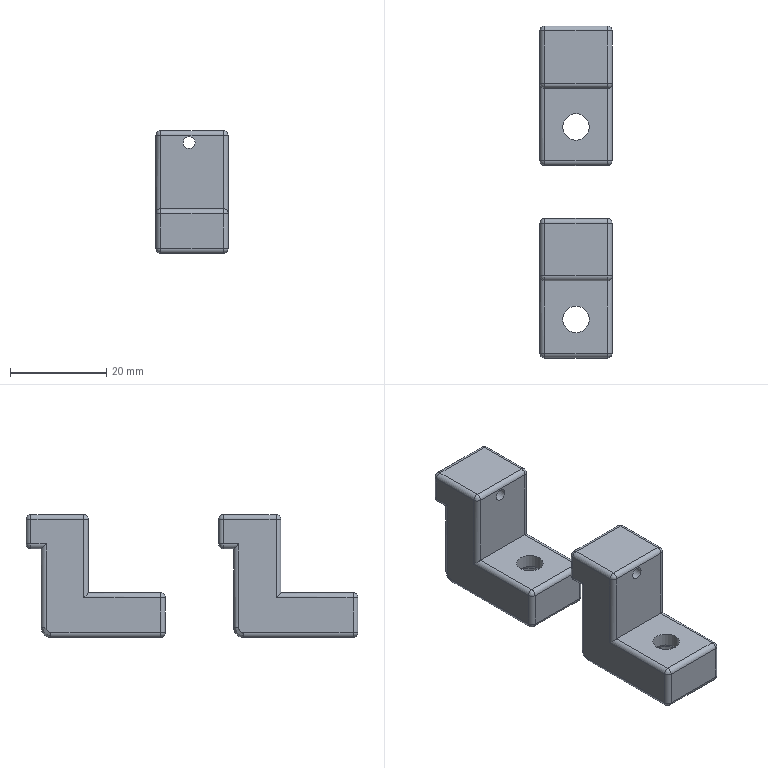CAM job | NX | 3-axis milling, drilling | part box 15 x 68.95 x 25.5 mm | stock box 20 x 73.95 x 30 mm
Tools:
number,name,description,diameter,corner_radius,flute_length,length,flutes
4,D4,平底铣刀-粗,4.0,0.0,25.0,75.0,2
6,D6,平底铣刀-粗,6.0,0.0,25.0,75.0,2
9,D10,平底铣刀-粗,10.0,0.0,35.0,75.0,2
7,D6-J,平底铣刀-精,6.0,0.0,25.0,75.0,2
18,D4R0.5,圆鼻刀-粗,4.0,0.5,50.0,75.0,2
1,D80R0.8飞刀,圆鼻刀-粗,80.0,0.8,50.0,75.0,2
1,D80R0.8飞刀-J,圆鼻刀-精,80.0,0.8,50.0,75.0,2
2,D6倒角刀,倒角刀,6.0,0.0,3.0,25.0,2
17,ZT5.5,钻头,5.5,0.0,35.0,50.0,2
Operations:
program,operation,operation_type,tool,method,geometry_group,spindle_rpm,surface_speed,feed_per_tooth,feed_cut,feed_plunge,cut_length_mm,path_length_mm,cut_time_min,machine_time_min
B,底壁铣飞面一刀开粗_COPY,VolumeBased25DMillingOperation,D80R0.8飞刀,分层开粗-切深K-步距G,W-B,2800.0,703.696,0.5357,3000.0,100.0,1594.679,3178.841,0.5316,0.69
B,底壁铣飞面一刀精光_COPY,VolumeBased25DMillingOperation,D80R0.8飞刀-J,侧刃精光-切深K-步距G,W-B,4000.0,1005.28,0.125,1000.0,100.0,176.99,212.99,0.177,0.1806
B,底壁铣分层开粗-中_COPY,VolumeBased25DMillingOperation,D10,分层开粗-切深K-步距G,W-B,8000.0,251.32,0.25,4000.0,100.0,7301.415,7478.472,1.825,1.843
B,等高螺旋爬面_COPY,ZLevelMilling,D4R0.5,等高爬面-切深K-步距G,W-B,7000.0,175.929,0.2857,4000.0,100.0,3123.524,3246.373,0.7809,0.7932
B,铣倒角_2,PlanarMilling,D6倒角刀,METHOD,W-B,8000.0,150.796,0.075,1200.0,100.0,35.589,225.483,0.0297,0.0486
B,底壁铣精光底面-中_COPY,VolumeBased25DMillingOperation,D6-J,精光步距切深关,W-B,7000.0,175.0,0.0536,1500.0,100.0,204.716,371.046,0.1365,0.1531
B,等高精光-中_COPY_1,ZLevelMilling,D6-J,侧刃精光-切深K-步距G,W-B,8000.0,150.792,0.0625,1000.0,100.0,123.039,377.209,0.123,0.1485
B,等高精光往复爬面_COPY_COPY_COPY_1,ZLevelMilling,D6-J,等高爬面-切深K-步距G,W-B,7000.0,87.965,0.3214,4500.0,100.0,1642.985,1808.549,0.3651,0.3817
A,顶面,FaceMilling,D80R0.8飞刀,侧刃精光-切深K-步距G,W-A,4000.0,1005.31,0.125,1000.0,100.0,162.95,198.95,0.1629,0.1665
A,外形粗_2,VolumeBased25DMillingOperation,D10,METHOD,W-A,8000.0,251.327,0.3125,5000.0,80.0,8042.542,8210.642,1.609,1.625
A,沉头孔打点-深0.8,Operation,D6倒角刀,NONE,W-A,8000.0,150.796,0.0312,500.0,90.0,3.6,88.213,0.0072,0.0157
A,沉头孔-钻孔0段,Operation,ZT5.5,NONE,W-A,1200.0,20.735,0.0625,150.0,90.0,27.805,136.622,0.1854,0.1962
A,底壁粗_1,VolumeBased25DMillingOperation,D4,METHOD,W-A,6000.0,56.549,0.0833,1000.0,100.0,6375.937,7477.18,6.376,6.486
A,铣孔开粗D6_1,CylinderMilling,D6,NONE,W-A,8000.0,150.796,0.075,1200.0,100.0,336.917,467.517,0.2808,0.2938
A,铣孔精光D6_1,CylinderMilling,D6,精光步距切深关,W-A,8000.0,150.796,0.0312,500.0,100.0,68.961,200.561,0.1379,0.1511
A,等高精光往复爬面_COPY,ZLevelMilling,D4R0.5,等高爬面-切深K-步距G,W-A,7000.0,87.965,0.3214,4500.0,100.0,3176.564,3261.452,0.7059,0.7144
A,等高精光往复爬面_COPY_COPY,ZLevelMilling,D4R0.5,等高爬面-切深K-步距G,W-A,7000.0,87.965,0.3214,4500.0,100.0,1874.539,1961.168,0.4166,0.4252
A,铣倒角_1,PlanarMilling,D6倒角刀,NONE,W-A,8000.0,150.796,0.05,800.0,100.0,80.502,196.93,0.1006,0.1123
A,等高精光-中_COPY,ZLevelMilling,D6-J,侧刃精光-切深K-步距G,W-A,8000.0,150.792,0.0625,1000.0,100.0,415.511,545.704,0.4155,0.4285
A,等高精光往复爬面_COPY_COPY_COPY,ZLevelMilling,D6-J,等高爬面-切深K-步距G,W-A,7000.0,87.965,0.3214,4500.0,100.0,5369.513,5522.32,1.193,1.208
A,外形半精_2,VolumeBased25DMillingOperation,D6-J,METHOD,W-A,8000.0,251.327,0.0625,1000.0,100.0,219.945,443.661,0.2199,0.2423